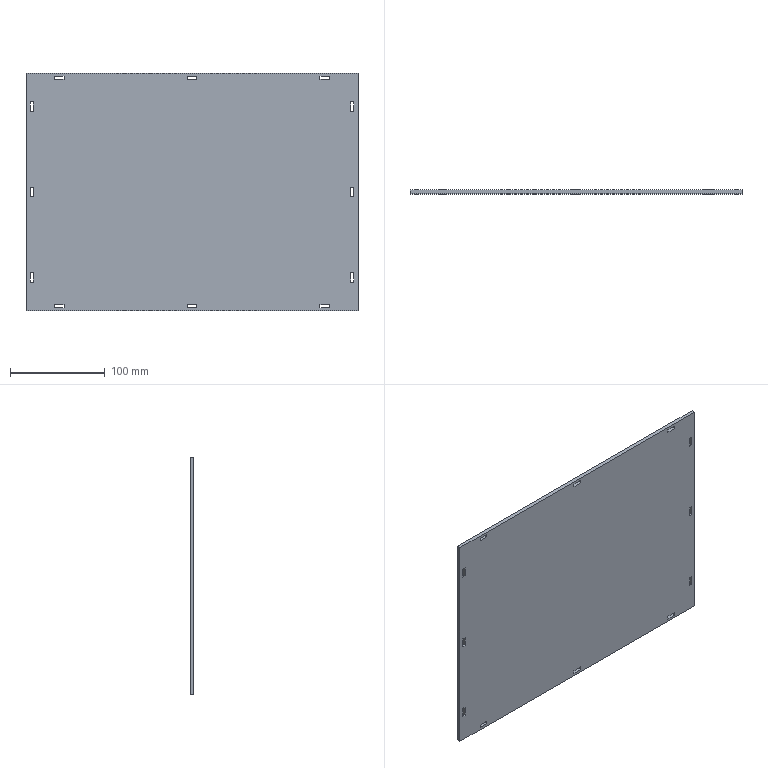Part | SolidWorks | features ICE 2, Extrusion 1 | 1 solid | 54 faces | box 350 x 4 x 250 mm | volume 348433 mm3 | plane 54